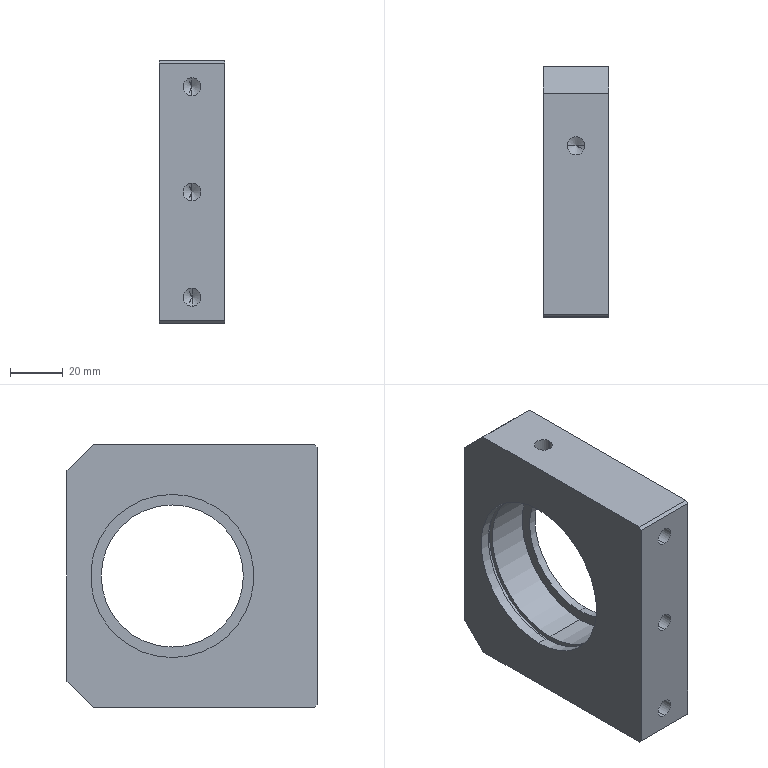Part | SolidWorks | features HoleWzd 3, ICE 3, Chamfer 2, Extrusion 1 | 1 solid | 41 faces | box 25 x 95 x 100 mm | volume 157637 mm3 | cylinder 18 | plane 13 | cone 10 | commonest cylinder face diameters 6.8 x10 62 x4 54 x2 65 x2
STEP:
#1=CARTESIAN_POINT('',(12.5,-27.75,43.4));
#2=VERTEX_POINT('',#1);
#3=CARTESIAN_POINT('',(12.5,-27.75,36.6));
#4=VERTEX_POINT('',#3);
#5=CARTESIAN_POINT('',(12.5,-27.75,40.));
#6=DIRECTION('',(0.,-1.,0.));
#7=DIRECTION('',(0.,0.,-1.));
#8=AXIS2_PLACEMENT_3D('',#5,#6,#7);
#9=CIRCLE('',#8,3.4);
#10=EDGE_CURVE('',#2,#4,#9,.T.);
#11=ORIENTED_EDGE('',*,*,#10,.F.);
#12=CARTESIAN_POINT('',(12.5,-47.5,43.4));
#13=VERTEX_POINT('',#12);
#14=CARTESIAN_POINT('',(12.5,-47.5,43.4));
#15=DIRECTION('',(0.,-1.,0.));
#16=VECTOR('',#15,1000.);
#17=LINE('',#14,#16);
#18=EDGE_CURVE('',#2,#13,#17,.T.);
#19=ORIENTED_EDGE('',*,*,#18,.T.);
#20=CARTESIAN_POINT('',(12.5,-47.5,36.6));
#21=VERTEX_POINT('',#20);
#22=CARTESIAN_POINT('',(12.5,-47.5,40.));
#23=DIRECTION('',(0.,-1.,0.));
#24=DIRECTION('',(0.,0.,-1.));
#25=AXIS2_PLACEMENT_3D('',#22,#23,#24);
#26=CIRCLE('',#25,3.4);
#27=EDGE_CURVE('',#13,#21,#26,.T.);
#28=ORIENTED_EDGE('',*,*,#27,.T.);
#29=CARTESIAN_POINT('',(12.5,-47.5,36.6));
#30=DIRECTION('',(0.,-1.,0.));
#31=VECTOR('',#30,1000.);
#32=LINE('',#29,#31);
#33=EDGE_CURVE('',#4,#21,#32,.T.);
#34=ORIENTED_EDGE('',*,*,#33,.F.);
#35=EDGE_LOOP('',(#11,#19,#28,#34));
#36=FACE_OUTER_BOUND('',#35,.T.);
#37=CARTESIAN_POINT('',(12.5,-47.5,40.));
#38=DIRECTION('',(0.,-1.,0.));
#39=DIRECTION('',(0.,0.,-1.));
#40=AXIS2_PLACEMENT_3D('',#37,#38,#39);
#41=CYLINDRICAL_SURFACE('',#40,3.4);
#42=ADVANCED_FACE('',(#36),#41,.F.);
#43=CARTESIAN_POINT('',(12.5,-25.707,40.));
#44=VERTEX_POINT('',#43);
#45=CARTESIAN_POINT('',(12.5,-27.75,36.6));
#46=DIRECTION('',(0.,-0.515,-0.8572));
#47=VECTOR('',#46,1000.);
#48=LINE('',#45,#47);
#49=EDGE_CURVE('',#44,#4,#48,.T.);
#50=ORIENTED_EDGE('',*,*,#49,.F.);
#51=CARTESIAN_POINT('',(12.5,-27.75,43.4));
#52=DIRECTION('',(0.,-0.515,0.8572));
#53=VECTOR('',#52,1000.);
#54=LINE('',#51,#53);
#55=EDGE_CURVE('',#44,#2,#54,.T.);
#56=ORIENTED_EDGE('',*,*,#55,.T.);
#57=ORIENTED_EDGE('',*,*,#10,.T.);
#58=EDGE_LOOP('',(#50,#56,#57));
#59=FACE_OUTER_BOUND('',#58,.T.);
#60=CARTESIAN_POINT('',(12.5,-27.75,40.));
#61=DIRECTION('',(0.,-1.,0.));
#62=DIRECTION('',(0.,0.,-1.));
#63=AXIS2_PLACEMENT_3D('',#60,#61,#62);
#64=CONICAL_SURFACE('',#63,3.4,1.03);
#65=ADVANCED_FACE('',(#59),#64,.F.);
#66=CARTESIAN_POINT('',(12.5,-27.75,3.4));
#67=VERTEX_POINT('',#66);
#68=CARTESIAN_POINT('',(12.5,-27.75,-3.4));
#69=VERTEX_POINT('',#68);
#70=CARTESIAN_POINT('',(12.5,-27.75,0.));
#71=DIRECTION('',(0.,-1.,0.));
#72=DIRECTION('',(0.,0.,-1.));
#73=AXIS2_PLACEMENT_3D('',#70,#71,#72);
#74=CIRCLE('',#73,3.4);
#75=EDGE_CURVE('',#67,#69,#74,.T.);
#76=ORIENTED_EDGE('',*,*,#75,.F.);
#77=CARTESIAN_POINT('',(12.5,-47.5,3.4));
#78=VERTEX_POINT('',#77);
#79=CARTESIAN_POINT('',(12.5,-47.5,3.4));
#80=DIRECTION('',(0.,-1.,0.));
#81=VECTOR('',#80,1000.);
#82=LINE('',#79,#81);
#83=EDGE_CURVE('',#67,#78,#82,.T.);
#84=ORIENTED_EDGE('',*,*,#83,.T.);
#85=CARTESIAN_POINT('',(12.5,-47.5,-3.4));
#86=VERTEX_POINT('',#85);
#87=CARTESIAN_POINT('',(12.5,-47.5,0.));
#88=DIRECTION('',(0.,-1.,0.));
#89=DIRECTION('',(0.,0.,-1.));
#90=AXIS2_PLACEMENT_3D('',#87,#88,#89);
#91=CIRCLE('',#90,3.4);
#92=EDGE_CURVE('',#78,#86,#91,.T.);
#93=ORIENTED_EDGE('',*,*,#92,.T.);
#94=CARTESIAN_POINT('',(12.5,-47.5,-3.4));
#95=DIRECTION('',(0.,-1.,0.));
#96=VECTOR('',#95,1000.);
#97=LINE('',#94,#96);
#98=EDGE_CURVE('',#69,#86,#97,.T.);
#99=ORIENTED_EDGE('',*,*,#98,.F.);
#100=EDGE_LOOP('',(#76,#84,#93,#99));
#101=FACE_OUTER_BOUND('',#100,.T.);
#102=CARTESIAN_POINT('',(12.5,-47.5,0.));
#103=DIRECTION('',(0.,-1.,0.));
#104=DIRECTION('',(0.,0.,-1.));
#105=AXIS2_PLACEMENT_3D('',#102,#103,#104);
#106=CYLINDRICAL_SURFACE('',#105,3.4);
#107=ADVANCED_FACE('',(#101),#106,.F.);
#108=CARTESIAN_POINT('',(12.5,-25.707,0.));
#109=VERTEX_POINT('',#108);
#110=CARTESIAN_POINT('',(12.5,-27.75,-3.4));
#111=DIRECTION('',(0.,-0.515,-0.8572));
#112=VECTOR('',#111,1000.);
#113=LINE('',#110,#112);
#114=EDGE_CURVE('',#109,#69,#113,.T.);
#115=ORIENTED_EDGE('',*,*,#114,.F.);
#116=CARTESIAN_POINT('',(12.5,-27.75,3.4));
#117=DIRECTION('',(0.,-0.515,0.8572));
#118=VECTOR('',#117,1000.);
#119=LINE('',#116,#118);
#120=EDGE_CURVE('',#109,#67,#119,.T.);
#121=ORIENTED_EDGE('',*,*,#120,.T.);
#122=ORIENTED_EDGE('',*,*,#75,.T.);
#123=EDGE_LOOP('',(#115,#121,#122));
#124=FACE_OUTER_BOUND('',#123,.T.);
#125=CARTESIAN_POINT('',(12.5,-27.75,0.));
#126=DIRECTION('',(0.,-1.,0.));
#127=DIRECTION('',(0.,0.,-1.));
#128=AXIS2_PLACEMENT_3D('',#125,#126,#127);
#129=CONICAL_SURFACE('',#128,3.4,1.03);
#130=ADVANCED_FACE('',(#124),#129,.F.);
#131=CARTESIAN_POINT('',(12.5,-27.75,-36.6));
#132=VERTEX_POINT('',#131);
#133=CARTESIAN_POINT('',(12.5,-27.75,-43.4));
#134=VERTEX_POINT('',#133);
#135=CARTESIAN_POINT('',(12.5,-27.75,-40.));
#136=DIRECTION('',(0.,-1.,0.));
#137=DIRECTION('',(0.,0.,-1.));
#138=AXIS2_PLACEMENT_3D('',#135,#136,#137);
#139=CIRCLE('',#138,3.4);
#140=EDGE_CURVE('',#132,#134,#139,.T.);
#141=ORIENTED_EDGE('',*,*,#140,.F.);
#142=CARTESIAN_POINT('',(12.5,-47.5,-36.6));
#143=VERTEX_POINT('',#142);
#144=CARTESIAN_POINT('',(12.5,-47.5,-36.6));
#145=DIRECTION('',(0.,-1.,0.));
#146=VECTOR('',#145,1000.);
#147=LINE('',#144,#146);
#148=EDGE_CURVE('',#132,#143,#147,.T.);
#149=ORIENTED_EDGE('',*,*,#148,.T.);
#150=CARTESIAN_POINT('',(12.5,-47.5,-43.4));
#151=VERTEX_POINT('',#150);
#152=CARTESIAN_POINT('',(12.5,-47.5,-40.));
#153=DIRECTION('',(0.,-1.,0.));
#154=DIRECTION('',(0.,0.,-1.));
#155=AXIS2_PLACEMENT_3D('',#152,#153,#154);
#156=CIRCLE('',#155,3.4);
#157=EDGE_CURVE('',#143,#151,#156,.T.);
#158=ORIENTED_EDGE('',*,*,#157,.T.);
#159=CARTESIAN_POINT('',(12.5,-47.5,-43.4));
#160=DIRECTION('',(0.,-1.,0.));
#161=VECTOR('',#160,1000.);
#162=LINE('',#159,#161);
#163=EDGE_CURVE('',#134,#151,#162,.T.);
#164=ORIENTED_EDGE('',*,*,#163,.F.);
#165=EDGE_LOOP('',(#141,#149,#158,#164));
#166=FACE_OUTER_BOUND('',#165,.T.);
#167=CARTESIAN_POINT('',(12.5,-47.5,-40.));
#168=DIRECTION('',(0.,-1.,0.));
#169=DIRECTION('',(0.,0.,-1.));
#170=AXIS2_PLACEMENT_3D('',#167,#168,#169);
#171=CYLINDRICAL_SURFACE('',#170,3.4);
#172=ADVANCED_FACE('',(#166),#171,.F.);
#173=CARTESIAN_POINT('',(12.5,-25.707,-40.));
#174=VERTEX_POINT('',#173);
#175=CARTESIAN_POINT('',(12.5,-27.75,-43.4));
#176=DIRECTION('',(0.,-0.515,-0.8572));
#177=VECTOR('',#176,1000.);
#178=LINE('',#175,#177);
#179=EDGE_CURVE('',#174,#134,#178,.T.);
#180=ORIENTED_EDGE('',*,*,#179,.F.);
#181=CARTESIAN_POINT('',(12.5,-27.75,-36.6));
#182=DIRECTION('',(0.,-0.515,0.8572));
#183=VECTOR('',#182,1000.);
#184=LINE('',#181,#183);
#185=EDGE_CURVE('',#174,#132,#184,.T.);
#186=ORIENTED_EDGE('',*,*,#185,.T.);
#187=ORIENTED_EDGE('',*,*,#140,.T.);
#188=EDGE_LOOP('',(#180,#186,#187));
#189=FACE_OUTER_BOUND('',#188,.T.);
#190=CARTESIAN_POINT('',(12.5,-27.75,-40.));
#191=DIRECTION('',(0.,-1.,0.));
#192=DIRECTION('',(0.,0.,-1.));
#193=AXIS2_PLACEMENT_3D('',#190,#191,#192);
#194=CONICAL_SURFACE('',#193,3.4,1.03);
#195=ADVANCED_FACE('',(#189),#194,.F.);
#196=CARTESIAN_POINT('',(12.5,14.1,-34.25));
#197=VERTEX_POINT('',#196);
#198=CARTESIAN_POINT('',(12.5,20.9,-34.25));
#199=VERTEX_POINT('',#198);
#200=CARTESIAN_POINT('',(12.5,17.5,-34.25));
#201=DIRECTION('',(0.,0.,-1.));
#202=DIRECTION('',(0.,1.,0.));
#203=AXIS2_PLACEMENT_3D('',#200,#201,#202);
#204=CIRCLE('',#203,3.4);
#205=EDGE_CURVE('',#197,#199,#204,.T.);
#206=ORIENTED_EDGE('',*,*,#205,.F.);
#207=CARTESIAN_POINT('',(12.5,14.1,-50.));
#208=VERTEX_POINT('',#207);
#209=CARTESIAN_POINT('',(12.5,14.1,-50.));
#210=DIRECTION('',(0.,0.,-1.));
#211=VECTOR('',#210,1000.);
#212=LINE('',#209,#211);
#213=EDGE_CURVE('',#197,#208,#212,.T.);
#214=ORIENTED_EDGE('',*,*,#213,.T.);
#215=CARTESIAN_POINT('',(12.5,20.9,-50.));
#216=VERTEX_POINT('',#215);
#217=CARTESIAN_POINT('',(12.5,17.5,-50.));
#218=DIRECTION('',(0.,0.,-1.));
#219=DIRECTION('',(0.,1.,0.));
#220=AXIS2_PLACEMENT_3D('',#217,#218,#219);
#221=CIRCLE('',#220,3.4);
#222=EDGE_CURVE('',#208,#216,#221,.T.);
#223=ORIENTED_EDGE('',*,*,#222,.T.);
#224=CARTESIAN_POINT('',(12.5,20.9,-50.));
#225=DIRECTION('',(0.,0.,-1.));
#226=VECTOR('',#225,1000.);
#227=LINE('',#224,#226);
#228=EDGE_CURVE('',#199,#216,#227,.T.);
#229=ORIENTED_EDGE('',*,*,#228,.F.);
#230=EDGE_LOOP('',(#206,#214,#223,#229));
#231=FACE_OUTER_BOUND('',#230,.T.);
#232=CARTESIAN_POINT('',(12.5,17.5,-50.));
#233=DIRECTION('',(0.,0.,-1.));
#234=DIRECTION('',(0.,1.,0.));
#235=AXIS2_PLACEMENT_3D('',#232,#233,#234);
#236=CYLINDRICAL_SURFACE('',#235,3.4);
#237=ADVANCED_FACE('',(#231),#236,.F.);
#238=CARTESIAN_POINT('',(12.5,17.5,-32.207));
#239=VERTEX_POINT('',#238);
#240=CARTESIAN_POINT('',(12.5,20.9,-34.25));
#241=DIRECTION('',(0.,0.8572,-0.515));
#242=VECTOR('',#241,1000.);
#243=LINE('',#240,#242);
#244=EDGE_CURVE('',#239,#199,#243,.T.);
#245=ORIENTED_EDGE('',*,*,#244,.F.);
#246=CARTESIAN_POINT('',(12.5,14.1,-34.25));
#247=DIRECTION('',(0.,-0.8572,-0.515));
#248=VECTOR('',#247,1000.);
#249=LINE('',#246,#248);
#250=EDGE_CURVE('',#239,#197,#249,.T.);
#251=ORIENTED_EDGE('',*,*,#250,.T.);
#252=ORIENTED_EDGE('',*,*,#205,.T.);
#253=EDGE_LOOP('',(#245,#251,#252));
#254=FACE_OUTER_BOUND('',#253,.T.);
#255=CARTESIAN_POINT('',(12.5,17.5,-34.25));
#256=DIRECTION('',(0.,0.,-1.));
#257=DIRECTION('',(0.,1.,0.));
#258=AXIS2_PLACEMENT_3D('',#255,#256,#257);
#259=CONICAL_SURFACE('',#258,3.4,1.03);
#260=ADVANCED_FACE('',(#254),#259,.F.);
#261=CARTESIAN_POINT('',(9.1,17.5,34.25));
#262=VERTEX_POINT('',#261);
#263=CARTESIAN_POINT('',(15.9,17.5,34.25));
#264=VERTEX_POINT('',#263);
#265=CARTESIAN_POINT('',(12.5,17.5,34.25));
#266=DIRECTION('',(0.,0.,1.));
#267=DIRECTION('',(1.,0.,0.));
#268=AXIS2_PLACEMENT_3D('',#265,#266,#267);
#269=CIRCLE('',#268,3.4);
#270=EDGE_CURVE('',#262,#264,#269,.T.);
#271=ORIENTED_EDGE('',*,*,#270,.F.);
#272=CARTESIAN_POINT('',(9.1,17.5,50.));
#273=VERTEX_POINT('',#272);
#274=CARTESIAN_POINT('',(9.1,17.5,50.));
#275=DIRECTION('',(0.,0.,1.));
#276=VECTOR('',#275,1000.);
#277=LINE('',#274,#276);
#278=EDGE_CURVE('',#262,#273,#277,.T.);
#279=ORIENTED_EDGE('',*,*,#278,.T.);
#280=CARTESIAN_POINT('',(15.9,17.5,50.));
#281=VERTEX_POINT('',#280);
#282=CARTESIAN_POINT('',(12.5,17.5,50.));
#283=DIRECTION('',(0.,0.,1.));
#284=DIRECTION('',(1.,0.,0.));
#285=AXIS2_PLACEMENT_3D('',#282,#283,#284);
#286=CIRCLE('',#285,3.4);
#287=EDGE_CURVE('',#273,#281,#286,.T.);
#288=ORIENTED_EDGE('',*,*,#287,.T.);
#289=CARTESIAN_POINT('',(15.9,17.5,50.));
#290=DIRECTION('',(0.,0.,1.));
#291=VECTOR('',#290,1000.);
#292=LINE('',#289,#291);
#293=EDGE_CURVE('',#264,#281,#292,.T.);
#294=ORIENTED_EDGE('',*,*,#293,.F.);
#295=EDGE_LOOP('',(#271,#279,#288,#294));
#296=FACE_OUTER_BOUND('',#295,.T.);
#297=CARTESIAN_POINT('',(12.5,17.5,50.));
#298=DIRECTION('',(0.,0.,1.));
#299=DIRECTION('',(1.,0.,0.));
#300=AXIS2_PLACEMENT_3D('',#297,#298,#299);
#301=CYLINDRICAL_SURFACE('',#300,3.4);
#302=ADVANCED_FACE('',(#296),#301,.F.);
#303=CARTESIAN_POINT('',(12.5,17.5,32.207));
#304=VERTEX_POINT('',#303);
#305=CARTESIAN_POINT('',(15.9,17.5,34.25));
#306=DIRECTION('',(0.8572,0.,0.515));
#307=VECTOR('',#306,1000.);
#308=LINE('',#305,#307);
#309=EDGE_CURVE('',#304,#264,#308,.T.);
#310=ORIENTED_EDGE('',*,*,#309,.F.);
#311=CARTESIAN_POINT('',(9.1,17.5,34.25));
#312=DIRECTION('',(-0.8572,0.,0.515));
#313=VECTOR('',#312,1000.);
#314=LINE('',#311,#313);
#315=EDGE_CURVE('',#304,#262,#314,.T.);
#316=ORIENTED_EDGE('',*,*,#315,.T.);
#317=ORIENTED_EDGE('',*,*,#270,.T.);
#318=EDGE_LOOP('',(#310,#316,#317));
#319=FACE_OUTER_BOUND('',#318,.T.);
#320=CARTESIAN_POINT('',(12.5,17.5,34.25));
#321=DIRECTION('',(0.,0.,1.));
#322=DIRECTION('',(1.,0.,0.));
#323=AXIS2_PLACEMENT_3D('',#320,#321,#322);
#324=CONICAL_SURFACE('',#323,3.4,1.03);
#325=ADVANCED_FACE('',(#319),#324,.F.);
#326=CARTESIAN_POINT('',(3.9,7.5,-32.5));
#327=VERTEX_POINT('',#326);
#328=CARTESIAN_POINT('',(3.9,7.5,32.5));
#329=VERTEX_POINT('',#328);
#330=CARTESIAN_POINT('',(3.9,7.5,0.));
#331=DIRECTION('',(-1.,0.,0.));
#332=DIRECTION('',(0.,0.,1.));
#333=AXIS2_PLACEMENT_3D('',#330,#331,#332);
#334=CIRCLE('',#333,32.5);
#335=EDGE_CURVE('',#327,#329,#334,.T.);
#336=ORIENTED_EDGE('',*,*,#335,.T.);
#337=CARTESIAN_POINT('',(6.,7.5,32.5));
#338=VERTEX_POINT('',#337);
#339=CARTESIAN_POINT('',(3.9,7.5,32.5));
#340=DIRECTION('',(1.,0.,0.));
#341=VECTOR('',#340,1000.);
#342=LINE('',#339,#341);
#343=EDGE_CURVE('',#329,#338,#342,.T.);
#344=ORIENTED_EDGE('',*,*,#343,.T.);
#345=CARTESIAN_POINT('',(6.,7.5,-32.5));
#346=VERTEX_POINT('',#345);
#347=CARTESIAN_POINT('',(6.,7.5,0.));
#348=DIRECTION('',(-1.,0.,0.));
#349=DIRECTION('',(0.,0.,1.));
#350=AXIS2_PLACEMENT_3D('',#347,#348,#349);
#351=CIRCLE('',#350,32.5);
#352=EDGE_CURVE('',#346,#338,#351,.T.);
#353=ORIENTED_EDGE('',*,*,#352,.F.);
#354=CARTESIAN_POINT('',(3.9,7.5,-32.5));
#355=DIRECTION('',(1.,0.,0.));
#356=VECTOR('',#355,1000.);
#357=LINE('',#354,#356);
#358=EDGE_CURVE('',#327,#346,#357,.T.);
#359=ORIENTED_EDGE('',*,*,#358,.F.);
#360=EDGE_LOOP('',(#336,#344,#353,#359));
#361=FACE_OUTER_BOUND('',#360,.T.);
#362=CARTESIAN_POINT('',(3.9,7.5,0.));
#363=DIRECTION('',(1.,0.,0.));
#364=DIRECTION('',(0.,0.,-1.));
#365=AXIS2_PLACEMENT_3D('',#362,#363,#364);
#366=CYLINDRICAL_SURFACE('',#365,32.5);
#367=ADVANCED_FACE('',(#361),#366,.F.);
#368=CARTESIAN_POINT('',(25.,7.5,-27.));
#369=VERTEX_POINT('',#368);
#370=CARTESIAN_POINT('',(25.,7.5,27.));
#371=VERTEX_POINT('',#370);
#372=CARTESIAN_POINT('',(25.,7.5,0.));
#373=DIRECTION('',(-1.,0.,0.));
#374=DIRECTION('',(0.,0.,1.));
#375=AXIS2_PLACEMENT_3D('',#372,#373,#374);
#376=CIRCLE('',#375,27.);
#377=EDGE_CURVE('',#369,#371,#376,.T.);
#378=ORIENTED_EDGE('',*,*,#377,.F.);
#379=CARTESIAN_POINT('',(22.,7.5,-27.));
#380=VERTEX_POINT('',#379);
#381=CARTESIAN_POINT('',(25.,7.5,-27.));
#382=DIRECTION('',(-1.,0.,0.));
#383=VECTOR('',#382,1000.);
#384=LINE('',#381,#383);
#385=EDGE_CURVE('',#369,#380,#384,.T.);
#386=ORIENTED_EDGE('',*,*,#385,.T.);
#387=CARTESIAN_POINT('',(22.,7.5,27.));
#388=VERTEX_POINT('',#387);
#389=CARTESIAN_POINT('',(22.,7.5,0.));
#390=DIRECTION('',(-1.,0.,0.));
#391=DIRECTION('',(0.,0.,1.));
#392=AXIS2_PLACEMENT_3D('',#389,#390,#391);
#393=CIRCLE('',#392,27.);
#394=EDGE_CURVE('',#380,#388,#393,.T.);
#395=ORIENTED_EDGE('',*,*,#394,.T.);
#396=CARTESIAN_POINT('',(25.,7.5,27.));
#397=DIRECTION('',(-1.,0.,0.));
#398=VECTOR('',#397,1000.);
#399=LINE('',#396,#398);
#400=EDGE_CURVE('',#371,#388,#399,.T.);
#401=ORIENTED_EDGE('',*,*,#400,.F.);
#402=EDGE_LOOP('',(#378,#386,#395,#401));
#403=FACE_OUTER_BOUND('',#402,.T.);
#404=CARTESIAN_POINT('',(25.,7.5,0.));
#405=DIRECTION('',(-1.,0.,0.));
#406=DIRECTION('',(0.,0.,1.));
#407=AXIS2_PLACEMENT_3D('',#404,#405,#406);
#408=CYLINDRICAL_SURFACE('',#407,27.);
#409=ADVANCED_FACE('',(#403),#408,.F.);
#410=CARTESIAN_POINT('',(3.9,7.5,31.));
#411=VERTEX_POINT('',#410);
#412=CARTESIAN_POINT('',(3.9,7.5,-31.));
#413=VERTEX_POINT('',#412);
#414=CARTESIAN_POINT('',(3.9,7.5,0.));
#415=DIRECTION('',(1.,0.,0.));
#416=DIRECTION('',(0.,0.,1.));
#417=AXIS2_PLACEMENT_3D('',#414,#415,#416);
#418=CIRCLE('',#417,31.);
#419=EDGE_CURVE('',#411,#413,#418,.T.);
#420=ORIENTED_EDGE('',*,*,#419,.T.);
#421=CARTESIAN_POINT('',(0.,7.5,-31.));
#422=VERTEX_POINT('',#421);
#423=CARTESIAN_POINT('',(22.,7.5,-31.));
#424=DIRECTION('',(-1.,0.,0.));
#425=VECTOR('',#424,1000.);
#426=LINE('',#423,#425);
#427=EDGE_CURVE('',#413,#422,#426,.T.);
#428=ORIENTED_EDGE('',*,*,#427,.T.);
#429=CARTESIAN_POINT('',(0.,7.5,31.));
#430=VERTEX_POINT('',#429);
#431=CARTESIAN_POINT('',(0.,7.5,0.));
#432=DIRECTION('',(-1.,0.,0.));
#433=DIRECTION('',(0.,0.,1.));
#434=AXIS2_PLACEMENT_3D('',#431,#432,#433);
#435=CIRCLE('',#434,31.);
#436=EDGE_CURVE('',#422,#430,#435,.T.);
#437=ORIENTED_EDGE('',*,*,#436,.T.);
#438=CARTESIAN_POINT('',(22.,7.5,31.));
#439=DIRECTION('',(-1.,0.,0.));
#440=VECTOR('',#439,1000.);
#441=LINE('',#438,#440);
#442=EDGE_CURVE('',#411,#430,#441,.T.);
#443=ORIENTED_EDGE('',*,*,#442,.F.);
#444=EDGE_LOOP('',(#420,#428,#437,#443));
#445=FACE_OUTER_BOUND('',#444,.T.);
#446=CARTESIAN_POINT('',(22.,7.5,0.));
#447=DIRECTION('',(-1.,0.,0.));
#448=DIRECTION('',(0.,0.,1.));
#449=AXIS2_PLACEMENT_3D('',#446,#447,#448);
#450=CYLINDRICAL_SURFACE('',#449,31.);
#451=ADVANCED_FACE('',(#445),#450,.F.);
#452=CARTESIAN_POINT('',(22.,7.5,-31.));
#453=VERTEX_POINT('',#452);
#454=CARTESIAN_POINT('',(22.,7.5,31.));
#455=VERTEX_POINT('',#454);
#456=CARTESIAN_POINT('',(22.,7.5,0.));
#457=DIRECTION('',(-1.,0.,0.));
#458=DIRECTION('',(0.,0.,1.));
#459=AXIS2_PLACEMENT_3D('',#456,#457,#458);
#460=CIRCLE('',#459,31.);
#461=EDGE_CURVE('',#453,#455,#460,.T.);
#462=ORIENTED_EDGE('',*,*,#461,.F.);
#463=CARTESIAN_POINT('',(6.,7.5,-31.));
#464=VERTEX_POINT('',#463);
#465=CARTESIAN_POINT('',(22.,7.5,-31.));
#466=DIRECTION('',(-1.,0.,0.));
#467=VECTOR('',#466,1000.);
#468=LINE('',#465,#467);
#469=EDGE_CURVE('',#453,#464,#468,.T.);
#470=ORIENTED_EDGE('',*,*,#469,.T.);
#471=CARTESIAN_POINT('',(6.,7.5,31.));
#472=VERTEX_POINT('',#471);
#473=CARTESIAN_POINT('',(6.,7.5,0.));
#474=DIRECTION('',(1.,0.,0.));
#475=DIRECTION('',(0.,0.,1.));
#476=AXIS2_PLACEMENT_3D('',#473,#474,#475);
#477=CIRCLE('',#476,31.);
#478=EDGE_CURVE('',#472,#464,#477,.T.);
#479=ORIENTED_EDGE('',*,*,#478,.F.);
#480=CARTESIAN_POINT('',(22.,7.5,31.));
#481=DIRECTION('',(-1.,0.,0.));
#482=VECTOR('',#481,1000.);
#483=LINE('',#480,#482);
#484=EDGE_CURVE('',#455,#472,#483,.T.);
#485=ORIENTED_EDGE('',*,*,#484,.F.);
#486=EDGE_LOOP('',(#462,#470,#479,#485));
#487=FACE_OUTER_BOUND('',#486,.T.);
#488=CARTESIAN_POINT('',(22.,7.5,0.));
#489=DIRECTION('',(-1.,0.,0.));
#490=DIRECTION('',(0.,0.,1.));
#491=AXIS2_PLACEMENT_3D('',#488,#489,#490);
#492=CYLINDRICAL_SURFACE('',#491,31.);
#493=ADVANCED_FACE('',(#487),#492,.F.);
#494=ORIENTED_EDGE('',*,*,#469,.F.);
#495=CARTESIAN_POINT('',(22.,7.5,0.));
#496=DIRECTION('',(-1.,0.,0.));
#497=DIRECTION('',(0.,0.,1.));
#498=AXIS2_PLACEMENT_3D('',#495,#496,#497);
#499=CIRCLE('',#498,31.);
#500=EDGE_CURVE('',#455,#453,#499,.T.);
#501=ORIENTED_EDGE('',*,*,#500,.F.);
#502=ORIENTED_EDGE('',*,*,#484,.T.);
#503=CARTESIAN_POINT('',(6.,7.5,0.));
#504=DIRECTION('',(1.,0.,0.));
#505=DIRECTION('',(0.,0.,1.));
#506=AXIS2_PLACEMENT_3D('',#503,#504,#505);
#507=CIRCLE('',#506,31.);
#508=EDGE_CURVE('',#464,#472,#507,.T.);
#509=ORIENTED_EDGE('',*,*,#508,.F.);
#510=EDGE_LOOP('',(#494,#501,#502,#509));
#511=FACE_OUTER_BOUND('',#510,.T.);
#512=CARTESIAN_POINT('',(22.,7.5,0.));
#513=DIRECTION('',(-1.,0.,0.));
#514=DIRECTION('',(0.,0.,1.));
#515=AXIS2_PLACEMENT_3D('',#512,#513,#514);
#516=CYLINDRICAL_SURFACE('',#515,31.);
#517=ADVANCED_FACE('',(#511),#516,.F.);
#518=CARTESIAN_POINT('',(12.5,17.5,-50.));
#519=DIRECTION('',(0.,0.,-1.));
#520=DIRECTION('',(0.,1.,0.));
#521=AXIS2_PLACEMENT_3D('',#518,#519,#520);
#522=CIRCLE('',#521,3.4);
#523=EDGE_CURVE('',#216,#208,#522,.T.);
#524=ORIENTED_EDGE('',*,*,#523,.F.);
#525=ORIENTED_EDGE('',*,*,#222,.F.);
#526=EDGE_LOOP('',(#524,#525));
#527=FACE_BOUND('',#526,.T.);
#528=CARTESIAN_POINT('',(25.,-46.5,-50.));
#529=VERTEX_POINT('',#528);
#530=CARTESIAN_POINT('',(25.,37.5,-50.));
#531=VERTEX_POINT('',#530);
#532=CARTESIAN_POINT('',(25.,47.5,-50.));
#533=DIRECTION('',(0.,1.,0.));
#534=VECTOR('',#533,1000.);
#535=LINE('',#532,#534);
#536=EDGE_CURVE('',#529,#531,#535,.T.);
#537=ORIENTED_EDGE('',*,*,#536,.F.);
#538=CARTESIAN_POINT('',(0.,-46.5,-50.));
#539=VERTEX_POINT('',#538);
#540=CARTESIAN_POINT('',(25.,-46.5,-50.));
#541=DIRECTION('',(-1.,0.,0.));
#542=VECTOR('',#541,1000.);
#543=LINE('',#540,#542);
#544=EDGE_CURVE('',#529,#539,#543,.T.);
#545=ORIENTED_EDGE('',*,*,#544,.T.);
#546=CARTESIAN_POINT('',(0.,37.5,-50.));
#547=VERTEX_POINT('',#546);
#548=CARTESIAN_POINT('',(0.,47.5,-50.));
#549=DIRECTION('',(0.,1.,0.));
#550=VECTOR('',#549,1000.);
#551=LINE('',#548,#550);
#552=EDGE_CURVE('',#539,#547,#551,.T.);
#553=ORIENTED_EDGE('',*,*,#552,.T.);
#554=CARTESIAN_POINT('',(25.,37.5,-50.));
#555=DIRECTION('',(1.,0.,0.));
#556=VECTOR('',#555,1000.);
#557=LINE('',#554,#556);
#558=EDGE_CURVE('',#547,#531,#557,.T.);
#559=ORIENTED_EDGE('',*,*,#558,.T.);
#560=EDGE_LOOP('',(#537,#545,#553,#559));
#561=FACE_OUTER_BOUND('',#560,.T.);
#562=CARTESIAN_POINT('',(25.,47.5,-50.));
#563=DIRECTION('',(0.,0.,1.));
#564=DIRECTION('',(0.,-1.,0.));
#565=AXIS2_PLACEMENT_3D('',#562,#563,#564);
#566=PLANE('',#565);
#567=ADVANCED_FACE('',(#527,#561),#566,.F.);
#568=CARTESIAN_POINT('',(25.,47.5,-40.));
#569=VERTEX_POINT('',#568);
#570=CARTESIAN_POINT('',(25.,47.5,40.));
#571=VERTEX_POINT('',#570);
#572=CARTESIAN_POINT('',(25.,47.5,50.));
#573=DIRECTION('',(0.,0.,1.));
#574=VECTOR('',#573,1000.);
#575=LINE('',#572,#574);
#576=EDGE_CURVE('',#569,#571,#575,.T.);
#577=ORIENTED_EDGE('',*,*,#576,.F.);
#578=CARTESIAN_POINT('',(0.,47.5,-40.));
#579=VERTEX_POINT('',#578);
#580=CARTESIAN_POINT('',(25.,47.5,-40.));
#581=DIRECTION('',(-1.,0.,0.));
#582=VECTOR('',#581,1000.);
#583=LINE('',#580,#582);
#584=EDGE_CURVE('',#569,#579,#583,.T.);
#585=ORIENTED_EDGE('',*,*,#584,.T.);
#586=CARTESIAN_POINT('',(0.,47.5,40.));
#587=VERTEX_POINT('',#586);
#588=CARTESIAN_POINT('',(0.,47.5,50.));
#589=DIRECTION('',(0.,0.,1.));
#590=VECTOR('',#589,1000.);
#591=LINE('',#588,#590);
#592=EDGE_CURVE('',#579,#587,#591,.T.);
#593=ORIENTED_EDGE('',*,*,#592,.T.);
#594=CARTESIAN_POINT('',(25.,47.5,40.));
#595=DIRECTION('',(1.,0.,0.));
#596=VECTOR('',#595,1000.);
#597=LINE('',#594,#596);
#598=EDGE_CURVE('',#587,#571,#597,.T.);
#599=ORIENTED_EDGE('',*,*,#598,.T.);
#600=EDGE_LOOP('',(#577,#585,#593,#599));
#601=FACE_OUTER_BOUND('',#600,.T.);
#602=CARTESIAN_POINT('',(25.,47.5,50.));
#603=DIRECTION('',(0.,-1.,0.));
#604=DIRECTION('',(0.,0.,-1.));
#605=AXIS2_PLACEMENT_3D('',#602,#603,#604);
#606=PLANE('',#605);
#607=ADVANCED_FACE('',(#601),#606,.F.);
#608=CARTESIAN_POINT('',(12.5,17.5,50.));
#609=DIRECTION('',(0.,0.,1.));
#610=DIRECTION('',(1.,0.,0.));
#611=AXIS2_PLACEMENT_3D('',#608,#609,#610);
#612=CIRCLE('',#611,3.4);
#613=EDGE_CURVE('',#281,#273,#612,.T.);
#614=ORIENTED_EDGE('',*,*,#613,.F.);
#615=ORIENTED_EDGE('',*,*,#287,.F.);
#616=EDGE_LOOP('',(#614,#615));
#617=FACE_BOUND('',#616,.T.);
#618=CARTESIAN_POINT('',(0.,37.5,50.));
#619=VERTEX_POINT('',#618);
#620=CARTESIAN_POINT('',(0.,-46.5,50.));
#621=VERTEX_POINT('',#620);
#622=CARTESIAN_POINT('',(0.,47.5,50.));
#623=DIRECTION('',(0.,-1.,0.));
#624=VECTOR('',#623,1000.);
#625=LINE('',#622,#624);
#626=EDGE_CURVE('',#619,#621,#625,.T.);
#627=ORIENTED_EDGE('',*,*,#626,.T.);
#628=CARTESIAN_POINT('',(25.,-46.5,50.));
#629=VERTEX_POINT('',#628);
#630=CARTESIAN_POINT('',(25.,-46.5,50.));
#631=DIRECTION('',(1.,0.,0.));
#632=VECTOR('',#631,1000.);
#633=LINE('',#630,#632);
#634=EDGE_CURVE('',#621,#629,#633,.T.);
#635=ORIENTED_EDGE('',*,*,#634,.T.);
#636=CARTESIAN_POINT('',(25.,37.5,50.));
#637=VERTEX_POINT('',#636);
#638=CARTESIAN_POINT('',(25.,47.5,50.));
#639=DIRECTION('',(0.,-1.,0.));
#640=VECTOR('',#639,1000.);
#641=LINE('',#638,#640);
#642=EDGE_CURVE('',#637,#629,#641,.T.);
#643=ORIENTED_EDGE('',*,*,#642,.F.);
#644=CARTESIAN_POINT('',(25.,37.5,50.));
#645=DIRECTION('',(-1.,0.,0.));
#646=VECTOR('',#645,1000.);
#647=LINE('',#644,#646);
#648=EDGE_CURVE('',#637,#619,#647,.T.);
#649=ORIENTED_EDGE('',*,*,#648,.T.);
#650=EDGE_LOOP('',(#627,#635,#643,#649));
#651=FACE_OUTER_BOUND('',#650,.T.);
#652=CARTESIAN_POINT('',(25.,47.5,50.));
#653=DIRECTION('',(0.,0.,-1.));
#654=DIRECTION('',(0.,1.,0.));
#655=AXIS2_PLACEMENT_3D('',#652,#653,#654);
#656=PLANE('',#655);
#657=ADVANCED_FACE('',(#617,#651),#656,.F.);
#658=CARTESIAN_POINT('',(12.5,-47.5,40.));
#659=DIRECTION('',(0.,-1.,0.));
#660=DIRECTION('',(0.,0.,-1.));
#661=AXIS2_PLACEMENT_3D('',#658,#659,#660);
#662=CIRCLE('',#661,3.4);
#663=EDGE_CURVE('',#21,#13,#662,.T.);
#664=ORIENTED_EDGE('',*,*,#663,.F.);
#665=ORIENTED_EDGE('',*,*,#27,.F.);
#666=EDGE_LOOP('',(#664,#665));
#667=FACE_BOUND('',#666,.T.);
#668=CARTESIAN_POINT('',(12.5,-47.5,0.));
#669=DIRECTION('',(0.,-1.,0.));
#670=DIRECTION('',(0.,0.,-1.));
#671=AXIS2_PLACEMENT_3D('',#668,#669,#670);
#672=CIRCLE('',#671,3.4);
#673=EDGE_CURVE('',#86,#78,#672,.T.);
#674=ORIENTED_EDGE('',*,*,#673,.F.);
#675=ORIENTED_EDGE('',*,*,#92,.F.);
#676=EDGE_LOOP('',(#674,#675));
#677=FACE_BOUND('',#676,.T.);
#678=CARTESIAN_POINT('',(12.5,-47.5,-40.));
#679=DIRECTION('',(0.,-1.,0.));
#680=DIRECTION('',(0.,0.,-1.));
#681=AXIS2_PLACEMENT_3D('',#678,#679,#680);
#682=CIRCLE('',#681,3.4);
#683=EDGE_CURVE('',#151,#143,#682,.T.);
#684=ORIENTED_EDGE('',*,*,#683,.F.);
#685=ORIENTED_EDGE('',*,*,#157,.F.);
#686=EDGE_LOOP('',(#684,#685));
#687=FACE_BOUND('',#686,.T.);
#688=CARTESIAN_POINT('',(0.,-47.5,49.));
#689=VERTEX_POINT('',#688);
#690=CARTESIAN_POINT('',(0.,-47.5,-49.));
#691=VERTEX_POINT('',#690);
#692=CARTESIAN_POINT('',(0.,-47.5,50.));
#693=DIRECTION('',(0.,0.,-1.));
#694=VECTOR('',#693,1000.);
#695=LINE('',#692,#694);
#696=EDGE_CURVE('',#689,#691,#695,.T.);
#697=ORIENTED_EDGE('',*,*,#696,.T.);
#698=CARTESIAN_POINT('',(25.,-47.5,-49.));
#699=VERTEX_POINT('',#698);
#700=CARTESIAN_POINT('',(25.,-47.5,-49.));
#701=DIRECTION('',(1.,0.,0.));
#702=VECTOR('',#701,1000.);
#703=LINE('',#700,#702);
#704=EDGE_CURVE('',#691,#699,#703,.T.);
#705=ORIENTED_EDGE('',*,*,#704,.T.);
#706=CARTESIAN_POINT('',(25.,-47.5,49.));
#707=VERTEX_POINT('',#706);
#708=CARTESIAN_POINT('',(25.,-47.5,50.));
#709=DIRECTION('',(0.,0.,-1.));
#710=VECTOR('',#709,1000.);
#711=LINE('',#708,#710);
#712=EDGE_CURVE('',#707,#699,#711,.T.);
#713=ORIENTED_EDGE('',*,*,#712,.F.);
#714=CARTESIAN_POINT('',(25.,-47.5,49.));
#715=DIRECTION('',(-1.,0.,0.));
#716=VECTOR('',#715,1000.);
#717=LINE('',#714,#716);
#718=EDGE_CURVE('',#707,#689,#717,.T.);
#719=ORIENTED_EDGE('',*,*,#718,.T.);
#720=EDGE_LOOP('',(#697,#705,#713,#719));
#721=FACE_OUTER_BOUND('',#720,.T.);
#722=CARTESIAN_POINT('',(25.,-47.5,50.));
#723=DIRECTION('',(0.,1.,0.));
#724=DIRECTION('',(0.,0.,1.));
#725=AXIS2_PLACEMENT_3D('',#722,#723,#724);
#726=PLANE('',#725);
#727=ADVANCED_FACE('',(#667,#677,#687,#721),#726,.F.);
#728=CARTESIAN_POINT('',(25.,7.5,0.));
#729=DIRECTION('',(-1.,0.,0.));
#730=DIRECTION('',(0.,0.,1.));
#731=AXIS2_PLACEMENT_3D('',#728,#729,#730);
#732=CIRCLE('',#731,27.);
#733=EDGE_CURVE('',#371,#369,#732,.T.);
#734=ORIENTED_EDGE('',*,*,#733,.T.);
#735=ORIENTED_EDGE('',*,*,#377,.T.);
#736=EDGE_LOOP('',(#734,#735));
#737=FACE_BOUND('',#736,.T.);
#738=ORIENTED_EDGE('',*,*,#712,.T.);
#739=CARTESIAN_POINT('',(25.,-48.25,-48.25));
#740=DIRECTION('',(0.,0.7071,-0.7071));
#741=VECTOR('',#740,1000.);
#742=LINE('',#739,#741);
#743=EDGE_CURVE('',#699,#529,#742,.T.);
#744=ORIENTED_EDGE('',*,*,#743,.T.);
#745=ORIENTED_EDGE('',*,*,#536,.T.);
#746=CARTESIAN_POINT('',(25.,43.75,-43.75));
#747=DIRECTION('',(0.,0.7071,0.7071));
#748=VECTOR('',#747,1000.);
#749=LINE('',#746,#748);
#750=EDGE_CURVE('',#531,#569,#749,.T.);
#751=ORIENTED_EDGE('',*,*,#750,.T.);
#752=ORIENTED_EDGE('',*,*,#576,.T.);
#753=CARTESIAN_POINT('',(25.,43.75,43.75));
#754=DIRECTION('',(0.,-0.7071,0.7071));
#755=VECTOR('',#754,1000.);
#756=LINE('',#753,#755);
#757=EDGE_CURVE('',#571,#637,#756,.T.);
#758=ORIENTED_EDGE('',*,*,#757,.T.);
#759=ORIENTED_EDGE('',*,*,#642,.T.);
#760=CARTESIAN_POINT('',(25.,-48.25,48.25));
#761=DIRECTION('',(0.,-0.7071,-0.7071));
#762=VECTOR('',#761,1000.);
#763=LINE('',#760,#762);
#764=EDGE_CURVE('',#629,#707,#763,.T.);
#765=ORIENTED_EDGE('',*,*,#764,.T.);
#766=EDGE_LOOP('',(#738,#744,#745,#751,#752,#758,#759,#765));
#767=FACE_OUTER_BOUND('',#766,.T.);
#768=CARTESIAN_POINT('',(25.,0.,0.));
#769=DIRECTION('',(1.,0.,0.));
#770=DIRECTION('',(0.,0.,-1.));
#771=AXIS2_PLACEMENT_3D('',#768,#769,#770);
#772=PLANE('',#771);
#773=ADVANCED_FACE('',(#737,#767),#772,.T.);
#774=CARTESIAN_POINT('',(0.,7.5,0.));
#775=DIRECTION('',(-1.,0.,0.));
#776=DIRECTION('',(0.,0.,1.));
#777=AXIS2_PLACEMENT_3D('',#774,#775,#776);
#778=CIRCLE('',#777,31.);
#779=EDGE_CURVE('',#430,#422,#778,.T.);
#780=ORIENTED_EDGE('',*,*,#779,.F.);
#781=ORIENTED_EDGE('',*,*,#436,.F.);
#782=EDGE_LOOP('',(#780,#781));
#783=FACE_BOUND('',#782,.T.);
#784=ORIENTED_EDGE('',*,*,#552,.F.);
#785=CARTESIAN_POINT('',(0.,-46.5,-50.));
#786=DIRECTION('',(0.,-0.7071,0.7071));
#787=VECTOR('',#786,1000.);
#788=LINE('',#785,#787);
#789=EDGE_CURVE('',#539,#691,#788,.T.);
#790=ORIENTED_EDGE('',*,*,#789,.T.);
#791=ORIENTED_EDGE('',*,*,#696,.F.);
#792=CARTESIAN_POINT('',(0.,-47.5,49.));
#793=DIRECTION('',(0.,0.7071,0.7071));
#794=VECTOR('',#793,1000.);
#795=LINE('',#792,#794);
#796=EDGE_CURVE('',#689,#621,#795,.T.);
#797=ORIENTED_EDGE('',*,*,#796,.T.);
#798=ORIENTED_EDGE('',*,*,#626,.F.);
#799=CARTESIAN_POINT('',(0.,37.5,50.));
#800=DIRECTION('',(0.,0.7071,-0.7071));
#801=VECTOR('',#800,1000.);
#802=LINE('',#799,#801);
#803=EDGE_CURVE('',#619,#587,#802,.T.);
#804=ORIENTED_EDGE('',*,*,#803,.T.);
#805=ORIENTED_EDGE('',*,*,#592,.F.);
#806=CARTESIAN_POINT('',(0.,47.5,-40.));
#807=DIRECTION('',(0.,-0.7071,-0.7071));
#808=VECTOR('',#807,1000.);
#809=LINE('',#806,#808);
#810=EDGE_CURVE('',#579,#547,#809,.T.);
#811=ORIENTED_EDGE('',*,*,#810,.T.);
#812=EDGE_LOOP('',(#784,#790,#791,#797,#798,#804,#805,#811));
#813=FACE_OUTER_BOUND('',#812,.T.);
#814=CARTESIAN_POINT('',(0.,0.,0.));
#815=DIRECTION('',(1.,0.,0.));
#816=DIRECTION('',(0.,0.,-1.));
#817=AXIS2_PLACEMENT_3D('',#814,#815,#816);
#818=PLANE('',#817);
#819=ADVANCED_FACE('',(#783,#813),#818,.F.);
#820=ORIENTED_EDGE('',*,*,#427,.F.);
#821=CARTESIAN_POINT('',(3.9,7.5,0.));
#822=DIRECTION('',(1.,0.,0.));
#823=DIRECTION('',(0.,0.,1.));
#824=AXIS2_PLACEMENT_3D('',#821,#822,#823);
#825=CIRCLE('',#824,31.);
#826=EDGE_CURVE('',#413,#411,#825,.T.);
#827=ORIENTED_EDGE('',*,*,#826,.T.);
#828=ORIENTED_EDGE('',*,*,#442,.T.);
#829=ORIENTED_EDGE('',*,*,#779,.T.);
#830=EDGE_LOOP('',(#820,#827,#828,#829));
#831=FACE_OUTER_BOUND('',#830,.T.);
#832=CARTESIAN_POINT('',(22.,7.5,0.));
#833=DIRECTION('',(-1.,0.,0.));
#834=DIRECTION('',(0.,0.,1.));
#835=AXIS2_PLACEMENT_3D('',#832,#833,#834);
#836=CYLINDRICAL_SURFACE('',#835,31.);
#837=ADVANCED_FACE('',(#831),#836,.F.);
#838=CARTESIAN_POINT('',(22.,7.5,0.));
#839=DIRECTION('',(-1.,0.,0.));
#840=DIRECTION('',(0.,0.,1.));
#841=AXIS2_PLACEMENT_3D('',#838,#839,#840);
#842=CIRCLE('',#841,27.);
#843=EDGE_CURVE('',#388,#380,#842,.T.);
#844=ORIENTED_EDGE('',*,*,#843,.F.);
#845=ORIENTED_EDGE('',*,*,#394,.F.);
#846=EDGE_LOOP('',(#844,#845));
#847=FACE_BOUND('',#846,.T.);
#848=ORIENTED_EDGE('',*,*,#500,.T.);
#849=ORIENTED_EDGE('',*,*,#461,.T.);
#850=EDGE_LOOP('',(#848,#849));
#851=FACE_OUTER_BOUND('',#850,.T.);
#852=CARTESIAN_POINT('',(22.,7.5,0.));
#853=DIRECTION('',(-1.,0.,0.));
#854=DIRECTION('',(0.,0.,1.));
#855=AXIS2_PLACEMENT_3D('',#852,#853,#854);
#856=PLANE('',#855);
#857=ADVANCED_FACE('',(#847,#851),#856,.T.);
#858=ORIENTED_EDGE('',*,*,#385,.F.);
#859=ORIENTED_EDGE('',*,*,#733,.F.);
#860=ORIENTED_EDGE('',*,*,#400,.T.);
#861=ORIENTED_EDGE('',*,*,#843,.T.);
#862=EDGE_LOOP('',(#858,#859,#860,#861));
#863=FACE_OUTER_BOUND('',#862,.T.);
#864=CARTESIAN_POINT('',(25.,7.5,0.));
#865=DIRECTION('',(-1.,0.,0.));
#866=DIRECTION('',(0.,0.,1.));
#867=AXIS2_PLACEMENT_3D('',#864,#865,#866);
#868=CYLINDRICAL_SURFACE('',#867,27.);
#869=ADVANCED_FACE('',(#863),#868,.F.);
#870=ORIENTED_EDGE('',*,*,#335,.F.);
#871=CARTESIAN_POINT('',(3.9,7.5,0.));
#872=DIRECTION('',(-1.,0.,0.));
#873=DIRECTION('',(0.,0.,1.));
#874=AXIS2_PLACEMENT_3D('',#871,#872,#873);
#875=CIRCLE('',#874,32.5);
#876=EDGE_CURVE('',#329,#327,#875,.T.);
#877=ORIENTED_EDGE('',*,*,#876,.F.);
#878=EDGE_LOOP('',(#870,#877));
#879=FACE_OUTER_BOUND('',#878,.T.);
#880=ORIENTED_EDGE('',*,*,#419,.F.);
#881=ORIENTED_EDGE('',*,*,#826,.F.);
#882=EDGE_LOOP('',(#880,#881));
#883=FACE_BOUND('',#882,.T.);
#884=CARTESIAN_POINT('',(3.9,7.5,0.));
#885=DIRECTION('',(-1.,0.,0.));
#886=DIRECTION('',(0.,0.,1.));
#887=AXIS2_PLACEMENT_3D('',#884,#885,#886);
#888=PLANE('',#887);
#889=ADVANCED_FACE('',(#879,#883),#888,.F.);
#890=ORIENTED_EDGE('',*,*,#352,.T.);
#891=CARTESIAN_POINT('',(6.,7.5,0.));
#892=DIRECTION('',(-1.,0.,0.));
#893=DIRECTION('',(0.,0.,1.));
#894=AXIS2_PLACEMENT_3D('',#891,#892,#893);
#895=CIRCLE('',#894,32.5);
#896=EDGE_CURVE('',#338,#346,#895,.T.);
#897=ORIENTED_EDGE('',*,*,#896,.T.);
#898=EDGE_LOOP('',(#890,#897));
#899=FACE_OUTER_BOUND('',#898,.T.);
#900=ORIENTED_EDGE('',*,*,#478,.T.);
#901=ORIENTED_EDGE('',*,*,#508,.T.);
#902=EDGE_LOOP('',(#900,#901));
#903=FACE_BOUND('',#902,.T.);
#904=CARTESIAN_POINT('',(6.,7.5,0.));
#905=DIRECTION('',(-1.,0.,0.));
#906=DIRECTION('',(0.,0.,1.));
#907=AXIS2_PLACEMENT_3D('',#904,#905,#906);
#908=PLANE('',#907);
#909=ADVANCED_FACE('',(#899,#903),#908,.T.);
#910=ORIENTED_EDGE('',*,*,#343,.F.);
#911=ORIENTED_EDGE('',*,*,#876,.T.);
#912=ORIENTED_EDGE('',*,*,#358,.T.);
#913=ORIENTED_EDGE('',*,*,#896,.F.);
#914=EDGE_LOOP('',(#910,#911,#912,#913));
#915=FACE_OUTER_BOUND('',#914,.T.);
#916=CARTESIAN_POINT('',(3.9,7.5,0.));
#917=DIRECTION('',(1.,0.,0.));
#918=DIRECTION('',(0.,0.,-1.));
#919=AXIS2_PLACEMENT_3D('',#916,#917,#918);
#920=CYLINDRICAL_SURFACE('',#919,32.5);
#921=ADVANCED_FACE('',(#915),#920,.F.);
#922=ORIENTED_EDGE('',*,*,#315,.F.);
#923=ORIENTED_EDGE('',*,*,#309,.T.);
#924=CARTESIAN_POINT('',(12.5,17.5,34.25));
#925=DIRECTION('',(0.,0.,1.));
#926=DIRECTION('',(1.,0.,0.));
#927=AXIS2_PLACEMENT_3D('',#924,#925,#926);
#928=CIRCLE('',#927,3.4);
#929=EDGE_CURVE('',#264,#262,#928,.T.);
#930=ORIENTED_EDGE('',*,*,#929,.T.);
#931=EDGE_LOOP('',(#922,#923,#930));
#932=FACE_OUTER_BOUND('',#931,.T.);
#933=CARTESIAN_POINT('',(12.5,17.5,34.25));
#934=DIRECTION('',(0.,0.,1.));
#935=DIRECTION('',(1.,0.,0.));
#936=AXIS2_PLACEMENT_3D('',#933,#934,#935);
#937=CONICAL_SURFACE('',#936,3.4,1.03);
#938=ADVANCED_FACE('',(#932),#937,.F.);
#939=ORIENTED_EDGE('',*,*,#278,.F.);
#940=ORIENTED_EDGE('',*,*,#929,.F.);
#941=ORIENTED_EDGE('',*,*,#293,.T.);
#942=ORIENTED_EDGE('',*,*,#613,.T.);
#943=EDGE_LOOP('',(#939,#940,#941,#942));
#944=FACE_OUTER_BOUND('',#943,.T.);
#945=CARTESIAN_POINT('',(12.5,17.5,50.));
#946=DIRECTION('',(0.,0.,1.));
#947=DIRECTION('',(1.,0.,0.));
#948=AXIS2_PLACEMENT_3D('',#945,#946,#947);
#949=CYLINDRICAL_SURFACE('',#948,3.4);
#950=ADVANCED_FACE('',(#944),#949,.F.);
#951=ORIENTED_EDGE('',*,*,#250,.F.);
#952=ORIENTED_EDGE('',*,*,#244,.T.);
#953=CARTESIAN_POINT('',(12.5,17.5,-34.25));
#954=DIRECTION('',(0.,0.,-1.));
#955=DIRECTION('',(0.,1.,0.));
#956=AXIS2_PLACEMENT_3D('',#953,#954,#955);
#957=CIRCLE('',#956,3.4);
#958=EDGE_CURVE('',#199,#197,#957,.T.);
#959=ORIENTED_EDGE('',*,*,#958,.T.);
#960=EDGE_LOOP('',(#951,#952,#959));
#961=FACE_OUTER_BOUND('',#960,.T.);
#962=CARTESIAN_POINT('',(12.5,17.5,-34.25));
#963=DIRECTION('',(0.,0.,-1.));
#964=DIRECTION('',(0.,1.,0.));
#965=AXIS2_PLACEMENT_3D('',#962,#963,#964);
#966=CONICAL_SURFACE('',#965,3.4,1.03);
#967=ADVANCED_FACE('',(#961),#966,.F.);
#968=ORIENTED_EDGE('',*,*,#213,.F.);
#969=ORIENTED_EDGE('',*,*,#958,.F.);
#970=ORIENTED_EDGE('',*,*,#228,.T.);
#971=ORIENTED_EDGE('',*,*,#523,.T.);
#972=EDGE_LOOP('',(#968,#969,#970,#971));
#973=FACE_OUTER_BOUND('',#972,.T.);
#974=CARTESIAN_POINT('',(12.5,17.5,-50.));
#975=DIRECTION('',(0.,0.,-1.));
#976=DIRECTION('',(0.,1.,0.));
#977=AXIS2_PLACEMENT_3D('',#974,#975,#976);
#978=CYLINDRICAL_SURFACE('',#977,3.4);
#979=ADVANCED_FACE('',(#973),#978,.F.);
#980=ORIENTED_EDGE('',*,*,#750,.F.);
#981=ORIENTED_EDGE('',*,*,#558,.F.);
#982=ORIENTED_EDGE('',*,*,#810,.F.);
#983=ORIENTED_EDGE('',*,*,#584,.F.);
#984=EDGE_LOOP('',(#980,#981,#982,#983));
#985=FACE_OUTER_BOUND('',#984,.T.);
#986=CARTESIAN_POINT('',(25.,47.5,-40.));
#987=DIRECTION('',(0.,-0.7071,0.7071));
#988=DIRECTION('',(-1.,0.,0.));
#989=AXIS2_PLACEMENT_3D('',#986,#987,#988);
#990=PLANE('',#989);
#991=ADVANCED_FACE('',(#985),#990,.F.);
#992=ORIENTED_EDGE('',*,*,#757,.F.);
#993=ORIENTED_EDGE('',*,*,#598,.F.);
#994=ORIENTED_EDGE('',*,*,#803,.F.);
#995=ORIENTED_EDGE('',*,*,#648,.F.);
#996=EDGE_LOOP('',(#992,#993,#994,#995));
#997=FACE_OUTER_BOUND('',#996,.T.);
#998=CARTESIAN_POINT('',(25.,37.5,50.));
#999=DIRECTION('',(0.,-0.7071,-0.7071));
#1000=DIRECTION('',(-1.,0.,0.));
#1001=AXIS2_PLACEMENT_3D('',#998,#999,#1000);
#1002=PLANE('',#1001);
#1003=ADVANCED_FACE('',(#997),#1002,.F.);
#1004=ORIENTED_EDGE('',*,*,#743,.F.);
#1005=ORIENTED_EDGE('',*,*,#704,.F.);
#1006=ORIENTED_EDGE('',*,*,#789,.F.);
#1007=ORIENTED_EDGE('',*,*,#544,.F.);
#1008=EDGE_LOOP('',(#1004,#1005,#1006,#1007));
#1009=FACE_OUTER_BOUND('',#1008,.T.);
#1010=CARTESIAN_POINT('',(25.,-46.5,-50.));
#1011=DIRECTION('',(0.,0.7071,0.7071));
#1012=DIRECTION('',(-1.,0.,0.));
#1013=AXIS2_PLACEMENT_3D('',#1010,#1011,#1012);
#1014=PLANE('',#1013);
#1015=ADVANCED_FACE('',(#1009),#1014,.F.);
#1016=ORIENTED_EDGE('',*,*,#764,.F.);
#1017=ORIENTED_EDGE('',*,*,#634,.F.);
#1018=ORIENTED_EDGE('',*,*,#796,.F.);
#1019=ORIENTED_EDGE('',*,*,#718,.F.);
#1020=EDGE_LOOP('',(#1016,#1017,#1018,#1019));
#1021=FACE_OUTER_BOUND('',#1020,.T.);
#1022=CARTESIAN_POINT('',(25.,-47.5,49.));
#1023=DIRECTION('',(0.,0.7071,-0.7071));
#1024=DIRECTION('',(-1.,0.,0.));
#1025=AXIS2_PLACEMENT_3D('',#1022,#1023,#1024);
#1026=PLANE('',#1025);
#1027=ADVANCED_FACE('',(#1021),#1026,.F.);
#1028=ORIENTED_EDGE('',*,*,#185,.F.);
#1029=ORIENTED_EDGE('',*,*,#179,.T.);
#1030=CARTESIAN_POINT('',(12.5,-27.75,-40.));
#1031=DIRECTION('',(0.,-1.,0.));
#1032=DIRECTION('',(0.,0.,-1.));
#1033=AXIS2_PLACEMENT_3D('',#1030,#1031,#1032);
#1034=CIRCLE('',#1033,3.4);
#1035=EDGE_CURVE('',#134,#132,#1034,.T.);
#1036=ORIENTED_EDGE('',*,*,#1035,.T.);
#1037=EDGE_LOOP('',(#1028,#1029,#1036));
#1038=FACE_OUTER_BOUND('',#1037,.T.);
#1039=CARTESIAN_POINT('',(12.5,-27.75,-40.));
#1040=DIRECTION('',(0.,-1.,0.));
#1041=DIRECTION('',(0.,0.,-1.));
#1042=AXIS2_PLACEMENT_3D('',#1039,#1040,#1041);
#1043=CONICAL_SURFACE('',#1042,3.4,1.03);
#1044=ADVANCED_FACE('',(#1038),#1043,.F.);
#1045=ORIENTED_EDGE('',*,*,#148,.F.);
#1046=ORIENTED_EDGE('',*,*,#1035,.F.);
#1047=ORIENTED_EDGE('',*,*,#163,.T.);
#1048=ORIENTED_EDGE('',*,*,#683,.T.);
#1049=EDGE_LOOP('',(#1045,#1046,#1047,#1048));
#1050=FACE_OUTER_BOUND('',#1049,.T.);
#1051=CARTESIAN_POINT('',(12.5,-47.5,-40.));
#1052=DIRECTION('',(0.,-1.,0.));
#1053=DIRECTION('',(0.,0.,-1.));
#1054=AXIS2_PLACEMENT_3D('',#1051,#1052,#1053);
#1055=CYLINDRICAL_SURFACE('',#1054,3.4);
#1056=ADVANCED_FACE('',(#1050),#1055,.F.);
#1057=ORIENTED_EDGE('',*,*,#120,.F.);
#1058=ORIENTED_EDGE('',*,*,#114,.T.);
#1059=CARTESIAN_POINT('',(12.5,-27.75,0.));
#1060=DIRECTION('',(0.,-1.,0.));
#1061=DIRECTION('',(0.,0.,-1.));
#1062=AXIS2_PLACEMENT_3D('',#1059,#1060,#1061);
#1063=CIRCLE('',#1062,3.4);
#1064=EDGE_CURVE('',#69,#67,#1063,.T.);
#1065=ORIENTED_EDGE('',*,*,#1064,.T.);
#1066=EDGE_LOOP('',(#1057,#1058,#1065));
#1067=FACE_OUTER_BOUND('',#1066,.T.);
#1068=CARTESIAN_POINT('',(12.5,-27.75,0.));
#1069=DIRECTION('',(0.,-1.,0.));
#1070=DIRECTION('',(0.,0.,-1.));
#1071=AXIS2_PLACEMENT_3D('',#1068,#1069,#1070);
#1072=CONICAL_SURFACE('',#1071,3.4,1.03);
#1073=ADVANCED_FACE('',(#1067),#1072,.F.);
#1074=ORIENTED_EDGE('',*,*,#83,.F.);
#1075=ORIENTED_EDGE('',*,*,#1064,.F.);
#1076=ORIENTED_EDGE('',*,*,#98,.T.);
#1077=ORIENTED_EDGE('',*,*,#673,.T.);
#1078=EDGE_LOOP('',(#1074,#1075,#1076,#1077));
#1079=FACE_OUTER_BOUND('',#1078,.T.);
#1080=CARTESIAN_POINT('',(12.5,-47.5,0.));
#1081=DIRECTION('',(0.,-1.,0.));
#1082=DIRECTION('',(0.,0.,-1.));
#1083=AXIS2_PLACEMENT_3D('',#1080,#1081,#1082);
#1084=CYLINDRICAL_SURFACE('',#1083,3.4);
#1085=ADVANCED_FACE('',(#1079),#1084,.F.);
#1086=ORIENTED_EDGE('',*,*,#55,.F.);
#1087=ORIENTED_EDGE('',*,*,#49,.T.);
#1088=CARTESIAN_POINT('',(12.5,-27.75,40.));
#1089=DIRECTION('',(0.,-1.,0.));
#1090=DIRECTION('',(0.,0.,-1.));
#1091=AXIS2_PLACEMENT_3D('',#1088,#1089,#1090);
#1092=CIRCLE('',#1091,3.4);
#1093=EDGE_CURVE('',#4,#2,#1092,.T.);
#1094=ORIENTED_EDGE('',*,*,#1093,.T.);
#1095=EDGE_LOOP('',(#1086,#1087,#1094));
#1096=FACE_OUTER_BOUND('',#1095,.T.);
#1097=CARTESIAN_POINT('',(12.5,-27.75,40.));
#1098=DIRECTION('',(0.,-1.,0.));
#1099=DIRECTION('',(0.,0.,-1.));
#1100=AXIS2_PLACEMENT_3D('',#1097,#1098,#1099);
#1101=CONICAL_SURFACE('',#1100,3.4,1.03);
#1102=ADVANCED_FACE('',(#1096),#1101,.F.);
#1103=ORIENTED_EDGE('',*,*,#18,.F.);
#1104=ORIENTED_EDGE('',*,*,#1093,.F.);
#1105=ORIENTED_EDGE('',*,*,#33,.T.);
#1106=ORIENTED_EDGE('',*,*,#663,.T.);
#1107=EDGE_LOOP('',(#1103,#1104,#1105,#1106));
#1108=FACE_OUTER_BOUND('',#1107,.T.);
#1109=CARTESIAN_POINT('',(12.5,-47.5,40.));
#1110=DIRECTION('',(0.,-1.,0.));
#1111=DIRECTION('',(0.,0.,-1.));
#1112=AXIS2_PLACEMENT_3D('',#1109,#1110,#1111);
#1113=CYLINDRICAL_SURFACE('',#1112,3.4);
#1114=ADVANCED_FACE('',(#1108),#1113,.F.);
#1115=CLOSED_SHELL('',(#42,#65,#107,#130,#172,#195,#237,#260,#302,#325,#367,#409,#451,#493,#517,#567,#607,#657,#727,#773,#819,#837,#857,#869,#889,#909,#921,#938,#950,#967,#979,#991,#1003,#1015,#1027,#1044,#1056,#1073,#1085,#1102,#1114));
#1116=MANIFOLD_SOLID_BREP('',#1115);
#1117=CARTESIAN_POINT('',(0.,0.,0.));
#1118=DIRECTION('',(0.,0.,1.));
#1119=DIRECTION('',(1.,0.,0.));
#1120=AXIS2_PLACEMENT_3D('',#1117,#1118,#1119);
#1121=(LENGTH_UNIT()NAMED_UNIT(*)SI_UNIT(.MILLI.,.METRE.));
#1122=UNCERTAINTY_MEASURE_WITH_UNIT(LENGTH_MEASURE(0.00001),#1121,'','');
#1123=(NAMED_UNIT(*)PLANE_ANGLE_UNIT()SI_UNIT($,.RADIAN.));
#1124=(NAMED_UNIT(*)SI_UNIT($,.STERADIAN.)SOLID_ANGLE_UNIT());
#1125=(GEOMETRIC_REPRESENTATION_CONTEXT(3)GLOBAL_UNCERTAINTY_ASSIGNED_CONTEXT((#1122))GLOBAL_UNIT_ASSIGNED_CONTEXT((#1121,#1123,#1124))REPRESENTATION_CONTEXT('',''));
#1126=ADVANCED_BREP_SHAPE_REPRESENTATION('',(#1116,#1120),#1125);